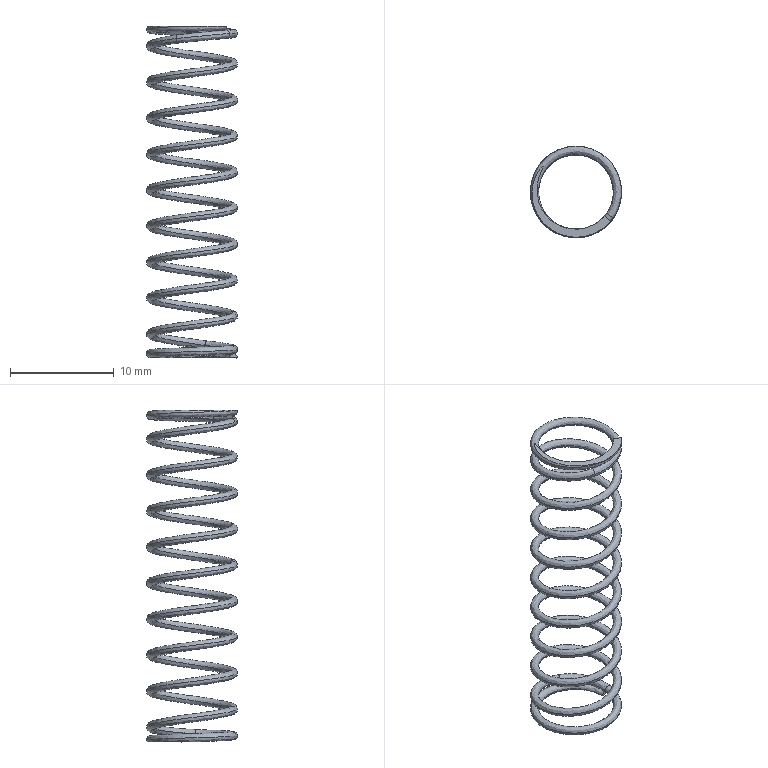Part | SolidWorks | features BaseBody 1 | 1 solid | 15 faces | box 8.799 x 8.797 x 32 mm | volume 125.702 mm3 | spline 11 | plane 4